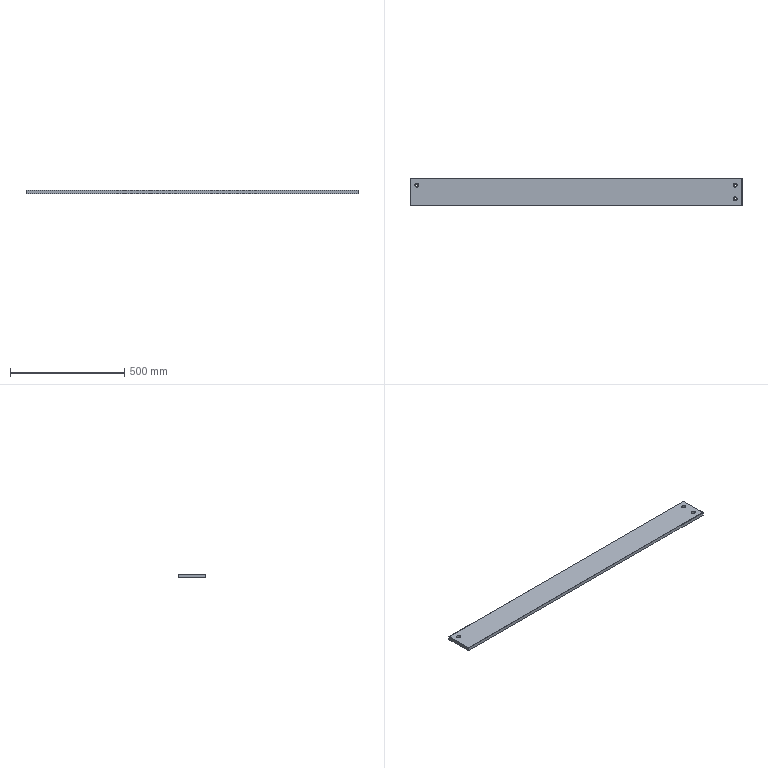Part | SolidWorks | features 3DProfileFeature 2, HoleWzd 2, Chamfer 1, Extrusion 1 | 1 solid | 25 faces | box 1453 x 120 x 15 mm | volume 2605469 mm3 | plane 13 | cylinder 12 | commonest cylinder face diameters 11 x6 18 x6
STEP:
#1=CARTESIAN_POINT('',(687.5,30.,-3.5));
#2=VERTEX_POINT('',#1);
#3=CARTESIAN_POINT('',(705.5,30.,-3.5));
#4=VERTEX_POINT('',#3);
#5=CARTESIAN_POINT('',(696.5,30.,-3.5));
#6=DIRECTION('',(0.,0.,1.));
#7=DIRECTION('',(1.,0.,0.));
#8=AXIS2_PLACEMENT_3D('',#5,#6,#7);
#9=CIRCLE('',#8,9.);
#10=EDGE_CURVE('',#2,#4,#9,.T.);
#11=ORIENTED_EDGE('',*,*,#10,.F.);
#12=CARTESIAN_POINT('',(687.5,30.,7.5));
#13=VERTEX_POINT('',#12);
#14=CARTESIAN_POINT('',(687.5,30.,7.5));
#15=DIRECTION('',(0.,0.,1.));
#16=VECTOR('',#15,1000.);
#17=LINE('',#14,#16);
#18=EDGE_CURVE('',#2,#13,#17,.T.);
#19=ORIENTED_EDGE('',*,*,#18,.T.);
#20=CARTESIAN_POINT('',(705.5,30.,7.5));
#21=VERTEX_POINT('',#20);
#22=CARTESIAN_POINT('',(696.5,30.,7.5));
#23=DIRECTION('',(0.,0.,1.));
#24=DIRECTION('',(1.,0.,0.));
#25=AXIS2_PLACEMENT_3D('',#22,#23,#24);
#26=CIRCLE('',#25,9.);
#27=EDGE_CURVE('',#13,#21,#26,.T.);
#28=ORIENTED_EDGE('',*,*,#27,.T.);
#29=CARTESIAN_POINT('',(705.5,30.,7.5));
#30=DIRECTION('',(0.,0.,1.));
#31=VECTOR('',#30,1000.);
#32=LINE('',#29,#31);
#33=EDGE_CURVE('',#4,#21,#32,.T.);
#34=ORIENTED_EDGE('',*,*,#33,.F.);
#35=EDGE_LOOP('',(#11,#19,#28,#34));
#36=FACE_OUTER_BOUND('',#35,.T.);
#37=CARTESIAN_POINT('',(696.5,30.,7.5));
#38=DIRECTION('',(0.,0.,1.));
#39=DIRECTION('',(1.,0.,0.));
#40=AXIS2_PLACEMENT_3D('',#37,#38,#39);
#41=CYLINDRICAL_SURFACE('',#40,9.);
#42=ADVANCED_FACE('',(#36),#41,.F.);
#43=CARTESIAN_POINT('',(691.,30.,-7.5));
#44=VERTEX_POINT('',#43);
#45=CARTESIAN_POINT('',(702.,30.,-7.5));
#46=VERTEX_POINT('',#45);
#47=CARTESIAN_POINT('',(696.5,30.,-7.5));
#48=DIRECTION('',(0.,0.,1.));
#49=DIRECTION('',(1.,0.,0.));
#50=AXIS2_PLACEMENT_3D('',#47,#48,#49);
#51=CIRCLE('',#50,5.5);
#52=EDGE_CURVE('',#44,#46,#51,.T.);
#53=ORIENTED_EDGE('',*,*,#52,.F.);
#54=CARTESIAN_POINT('',(691.,30.,-3.5));
#55=VERTEX_POINT('',#54);
#56=CARTESIAN_POINT('',(691.,30.,7.5));
#57=DIRECTION('',(0.,0.,1.));
#58=VECTOR('',#57,1000.);
#59=LINE('',#56,#58);
#60=EDGE_CURVE('',#44,#55,#59,.T.);
#61=ORIENTED_EDGE('',*,*,#60,.T.);
#62=CARTESIAN_POINT('',(702.,30.,-3.5));
#63=VERTEX_POINT('',#62);
#64=CARTESIAN_POINT('',(696.5,30.,-3.5));
#65=DIRECTION('',(0.,0.,1.));
#66=DIRECTION('',(1.,0.,0.));
#67=AXIS2_PLACEMENT_3D('',#64,#65,#66);
#68=CIRCLE('',#67,5.5);
#69=EDGE_CURVE('',#55,#63,#68,.T.);
#70=ORIENTED_EDGE('',*,*,#69,.T.);
#71=CARTESIAN_POINT('',(702.,30.,7.5));
#72=DIRECTION('',(0.,0.,1.));
#73=VECTOR('',#72,1000.);
#74=LINE('',#71,#73);
#75=EDGE_CURVE('',#46,#63,#74,.T.);
#76=ORIENTED_EDGE('',*,*,#75,.F.);
#77=EDGE_LOOP('',(#53,#61,#70,#76));
#78=FACE_OUTER_BOUND('',#77,.T.);
#79=CARTESIAN_POINT('',(696.5,30.,7.5));
#80=DIRECTION('',(0.,0.,1.));
#81=DIRECTION('',(1.,0.,0.));
#82=AXIS2_PLACEMENT_3D('',#79,#80,#81);
#83=CYLINDRICAL_SURFACE('',#82,5.5);
#84=ADVANCED_FACE('',(#78),#83,.F.);
#85=CARTESIAN_POINT('',(687.5,-30.,-3.5));
#86=VERTEX_POINT('',#85);
#87=CARTESIAN_POINT('',(705.5,-30.,-3.5));
#88=VERTEX_POINT('',#87);
#89=CARTESIAN_POINT('',(696.5,-30.,-3.5));
#90=DIRECTION('',(0.,0.,1.));
#91=DIRECTION('',(1.,0.,0.));
#92=AXIS2_PLACEMENT_3D('',#89,#90,#91);
#93=CIRCLE('',#92,9.);
#94=EDGE_CURVE('',#86,#88,#93,.T.);
#95=ORIENTED_EDGE('',*,*,#94,.F.);
#96=CARTESIAN_POINT('',(687.5,-30.,7.5));
#97=VERTEX_POINT('',#96);
#98=CARTESIAN_POINT('',(687.5,-30.,7.5));
#99=DIRECTION('',(0.,0.,1.));
#100=VECTOR('',#99,1000.);
#101=LINE('',#98,#100);
#102=EDGE_CURVE('',#86,#97,#101,.T.);
#103=ORIENTED_EDGE('',*,*,#102,.T.);
#104=CARTESIAN_POINT('',(705.5,-30.,7.5));
#105=VERTEX_POINT('',#104);
#106=CARTESIAN_POINT('',(696.5,-30.,7.5));
#107=DIRECTION('',(0.,0.,1.));
#108=DIRECTION('',(1.,0.,0.));
#109=AXIS2_PLACEMENT_3D('',#106,#107,#108);
#110=CIRCLE('',#109,9.);
#111=EDGE_CURVE('',#97,#105,#110,.T.);
#112=ORIENTED_EDGE('',*,*,#111,.T.);
#113=CARTESIAN_POINT('',(705.5,-30.,7.5));
#114=DIRECTION('',(0.,0.,1.));
#115=VECTOR('',#114,1000.);
#116=LINE('',#113,#115);
#117=EDGE_CURVE('',#88,#105,#116,.T.);
#118=ORIENTED_EDGE('',*,*,#117,.F.);
#119=EDGE_LOOP('',(#95,#103,#112,#118));
#120=FACE_OUTER_BOUND('',#119,.T.);
#121=CARTESIAN_POINT('',(696.5,-30.,7.5));
#122=DIRECTION('',(0.,0.,1.));
#123=DIRECTION('',(1.,0.,0.));
#124=AXIS2_PLACEMENT_3D('',#121,#122,#123);
#125=CYLINDRICAL_SURFACE('',#124,9.);
#126=ADVANCED_FACE('',(#120),#125,.F.);
#127=CARTESIAN_POINT('',(691.,-30.,-7.5));
#128=VERTEX_POINT('',#127);
#129=CARTESIAN_POINT('',(702.,-30.,-7.5));
#130=VERTEX_POINT('',#129);
#131=CARTESIAN_POINT('',(696.5,-30.,-7.5));
#132=DIRECTION('',(0.,0.,1.));
#133=DIRECTION('',(1.,0.,0.));
#134=AXIS2_PLACEMENT_3D('',#131,#132,#133);
#135=CIRCLE('',#134,5.5);
#136=EDGE_CURVE('',#128,#130,#135,.T.);
#137=ORIENTED_EDGE('',*,*,#136,.F.);
#138=CARTESIAN_POINT('',(691.,-30.,-3.5));
#139=VERTEX_POINT('',#138);
#140=CARTESIAN_POINT('',(691.,-30.,7.5));
#141=DIRECTION('',(0.,0.,1.));
#142=VECTOR('',#141,1000.);
#143=LINE('',#140,#142);
#144=EDGE_CURVE('',#128,#139,#143,.T.);
#145=ORIENTED_EDGE('',*,*,#144,.T.);
#146=CARTESIAN_POINT('',(702.,-30.,-3.5));
#147=VERTEX_POINT('',#146);
#148=CARTESIAN_POINT('',(696.5,-30.,-3.5));
#149=DIRECTION('',(0.,0.,1.));
#150=DIRECTION('',(1.,0.,0.));
#151=AXIS2_PLACEMENT_3D('',#148,#149,#150);
#152=CIRCLE('',#151,5.5);
#153=EDGE_CURVE('',#139,#147,#152,.T.);
#154=ORIENTED_EDGE('',*,*,#153,.T.);
#155=CARTESIAN_POINT('',(702.,-30.,7.5));
#156=DIRECTION('',(0.,0.,1.));
#157=VECTOR('',#156,1000.);
#158=LINE('',#155,#157);
#159=EDGE_CURVE('',#130,#147,#158,.T.);
#160=ORIENTED_EDGE('',*,*,#159,.F.);
#161=EDGE_LOOP('',(#137,#145,#154,#160));
#162=FACE_OUTER_BOUND('',#161,.T.);
#163=CARTESIAN_POINT('',(696.5,-30.,7.5));
#164=DIRECTION('',(0.,0.,1.));
#165=DIRECTION('',(1.,0.,0.));
#166=AXIS2_PLACEMENT_3D('',#163,#164,#165);
#167=CYLINDRICAL_SURFACE('',#166,5.5);
#168=ADVANCED_FACE('',(#162),#167,.F.);
#169=CARTESIAN_POINT('',(-705.5,30.,-3.5));
#170=VERTEX_POINT('',#169);
#171=CARTESIAN_POINT('',(-687.5,30.,-3.5));
#172=VERTEX_POINT('',#171);
#173=CARTESIAN_POINT('',(-696.5,30.,-3.5));
#174=DIRECTION('',(0.,0.,1.));
#175=DIRECTION('',(1.,0.,0.));
#176=AXIS2_PLACEMENT_3D('',#173,#174,#175);
#177=CIRCLE('',#176,9.);
#178=EDGE_CURVE('',#170,#172,#177,.T.);
#179=ORIENTED_EDGE('',*,*,#178,.F.);
#180=CARTESIAN_POINT('',(-705.5,30.,7.5));
#181=VERTEX_POINT('',#180);
#182=CARTESIAN_POINT('',(-705.5,30.,7.5));
#183=DIRECTION('',(0.,0.,1.));
#184=VECTOR('',#183,1000.);
#185=LINE('',#182,#184);
#186=EDGE_CURVE('',#170,#181,#185,.T.);
#187=ORIENTED_EDGE('',*,*,#186,.T.);
#188=CARTESIAN_POINT('',(-687.5,30.,7.5));
#189=VERTEX_POINT('',#188);
#190=CARTESIAN_POINT('',(-696.5,30.,7.5));
#191=DIRECTION('',(0.,0.,1.));
#192=DIRECTION('',(1.,0.,0.));
#193=AXIS2_PLACEMENT_3D('',#190,#191,#192);
#194=CIRCLE('',#193,9.);
#195=EDGE_CURVE('',#181,#189,#194,.T.);
#196=ORIENTED_EDGE('',*,*,#195,.T.);
#197=CARTESIAN_POINT('',(-687.5,30.,7.5));
#198=DIRECTION('',(0.,0.,1.));
#199=VECTOR('',#198,1000.);
#200=LINE('',#197,#199);
#201=EDGE_CURVE('',#172,#189,#200,.T.);
#202=ORIENTED_EDGE('',*,*,#201,.F.);
#203=EDGE_LOOP('',(#179,#187,#196,#202));
#204=FACE_OUTER_BOUND('',#203,.T.);
#205=CARTESIAN_POINT('',(-696.5,30.,7.5));
#206=DIRECTION('',(0.,0.,1.));
#207=DIRECTION('',(1.,0.,0.));
#208=AXIS2_PLACEMENT_3D('',#205,#206,#207);
#209=CYLINDRICAL_SURFACE('',#208,9.);
#210=ADVANCED_FACE('',(#204),#209,.F.);
#211=CARTESIAN_POINT('',(-702.,30.,-7.5));
#212=VERTEX_POINT('',#211);
#213=CARTESIAN_POINT('',(-691.,30.,-7.5));
#214=VERTEX_POINT('',#213);
#215=CARTESIAN_POINT('',(-696.5,30.,-7.5));
#216=DIRECTION('',(0.,0.,1.));
#217=DIRECTION('',(1.,0.,0.));
#218=AXIS2_PLACEMENT_3D('',#215,#216,#217);
#219=CIRCLE('',#218,5.5);
#220=EDGE_CURVE('',#212,#214,#219,.T.);
#221=ORIENTED_EDGE('',*,*,#220,.F.);
#222=CARTESIAN_POINT('',(-702.,30.,-3.5));
#223=VERTEX_POINT('',#222);
#224=CARTESIAN_POINT('',(-702.,30.,7.5));
#225=DIRECTION('',(0.,0.,1.));
#226=VECTOR('',#225,1000.);
#227=LINE('',#224,#226);
#228=EDGE_CURVE('',#212,#223,#227,.T.);
#229=ORIENTED_EDGE('',*,*,#228,.T.);
#230=CARTESIAN_POINT('',(-691.,30.,-3.5));
#231=VERTEX_POINT('',#230);
#232=CARTESIAN_POINT('',(-696.5,30.,-3.5));
#233=DIRECTION('',(0.,0.,1.));
#234=DIRECTION('',(1.,0.,0.));
#235=AXIS2_PLACEMENT_3D('',#232,#233,#234);
#236=CIRCLE('',#235,5.5);
#237=EDGE_CURVE('',#223,#231,#236,.T.);
#238=ORIENTED_EDGE('',*,*,#237,.T.);
#239=CARTESIAN_POINT('',(-691.,30.,7.5));
#240=DIRECTION('',(0.,0.,1.));
#241=VECTOR('',#240,1000.);
#242=LINE('',#239,#241);
#243=EDGE_CURVE('',#214,#231,#242,.T.);
#244=ORIENTED_EDGE('',*,*,#243,.F.);
#245=EDGE_LOOP('',(#221,#229,#238,#244));
#246=FACE_OUTER_BOUND('',#245,.T.);
#247=CARTESIAN_POINT('',(-696.5,30.,7.5));
#248=DIRECTION('',(0.,0.,1.));
#249=DIRECTION('',(1.,0.,0.));
#250=AXIS2_PLACEMENT_3D('',#247,#248,#249);
#251=CYLINDRICAL_SURFACE('',#250,5.5);
#252=ADVANCED_FACE('',(#246),#251,.F.);
#253=CARTESIAN_POINT('',(726.5,60.,7.));
#254=VERTEX_POINT('',#253);
#255=CARTESIAN_POINT('',(726.5,60.,-7.5));
#256=VERTEX_POINT('',#255);
#257=CARTESIAN_POINT('',(726.5,60.,7.5));
#258=DIRECTION('',(0.,0.,-1.));
#259=VECTOR('',#258,1000.);
#260=LINE('',#257,#259);
#261=EDGE_CURVE('',#254,#256,#260,.T.);
#262=ORIENTED_EDGE('',*,*,#261,.F.);
#263=CARTESIAN_POINT('',(726.5,-60.,7.));
#264=VERTEX_POINT('',#263);
#265=CARTESIAN_POINT('',(726.5,-60.,7.));
#266=DIRECTION('',(0.,-1.,0.));
#267=VECTOR('',#266,1000.);
#268=LINE('',#265,#267);
#269=EDGE_CURVE('',#254,#264,#268,.T.);
#270=ORIENTED_EDGE('',*,*,#269,.T.);
#271=CARTESIAN_POINT('',(726.5,-60.,-7.5));
#272=VERTEX_POINT('',#271);
#273=CARTESIAN_POINT('',(726.5,-60.,7.5));
#274=DIRECTION('',(0.,0.,-1.));
#275=VECTOR('',#274,1000.);
#276=LINE('',#273,#275);
#277=EDGE_CURVE('',#264,#272,#276,.T.);
#278=ORIENTED_EDGE('',*,*,#277,.T.);
#279=CARTESIAN_POINT('',(726.5,60.,-7.5));
#280=DIRECTION('',(0.,1.,0.));
#281=VECTOR('',#280,1000.);
#282=LINE('',#279,#281);
#283=EDGE_CURVE('',#272,#256,#282,.T.);
#284=ORIENTED_EDGE('',*,*,#283,.T.);
#285=EDGE_LOOP('',(#262,#270,#278,#284));
#286=FACE_OUTER_BOUND('',#285,.T.);
#287=CARTESIAN_POINT('',(726.5,60.,7.5));
#288=DIRECTION('',(-1.,0.,0.));
#289=DIRECTION('',(0.,0.,1.));
#290=AXIS2_PLACEMENT_3D('',#287,#288,#289);
#291=PLANE('',#290);
#292=ADVANCED_FACE('',(#286),#291,.F.);
#293=CARTESIAN_POINT('',(-726.5,60.,7.));
#294=VERTEX_POINT('',#293);
#295=CARTESIAN_POINT('',(-726.5,60.,-7.5));
#296=VERTEX_POINT('',#295);
#297=CARTESIAN_POINT('',(-726.5,60.,7.5));
#298=DIRECTION('',(0.,0.,-1.));
#299=VECTOR('',#298,1000.);
#300=LINE('',#297,#299);
#301=EDGE_CURVE('',#294,#296,#300,.T.);
#302=ORIENTED_EDGE('',*,*,#301,.F.);
#303=CARTESIAN_POINT('',(726.5,60.,7.));
#304=DIRECTION('',(1.,0.,0.));
#305=VECTOR('',#304,1000.);
#306=LINE('',#303,#305);
#307=EDGE_CURVE('',#294,#254,#306,.T.);
#308=ORIENTED_EDGE('',*,*,#307,.T.);
#309=ORIENTED_EDGE('',*,*,#261,.T.);
#310=CARTESIAN_POINT('',(-726.5,60.,-7.5));
#311=DIRECTION('',(-1.,0.,0.));
#312=VECTOR('',#311,1000.);
#313=LINE('',#310,#312);
#314=EDGE_CURVE('',#256,#296,#313,.T.);
#315=ORIENTED_EDGE('',*,*,#314,.T.);
#316=EDGE_LOOP('',(#302,#308,#309,#315));
#317=FACE_OUTER_BOUND('',#316,.T.);
#318=CARTESIAN_POINT('',(-726.5,60.,7.5));
#319=DIRECTION('',(0.,-1.,0.));
#320=DIRECTION('',(0.,0.,-1.));
#321=AXIS2_PLACEMENT_3D('',#318,#319,#320);
#322=PLANE('',#321);
#323=ADVANCED_FACE('',(#317),#322,.F.);
#324=CARTESIAN_POINT('',(-726.5,-60.,7.));
#325=VERTEX_POINT('',#324);
#326=CARTESIAN_POINT('',(-726.5,-60.,-7.5));
#327=VERTEX_POINT('',#326);
#328=CARTESIAN_POINT('',(-726.5,-60.,7.5));
#329=DIRECTION('',(0.,0.,-1.));
#330=VECTOR('',#329,1000.);
#331=LINE('',#328,#330);
#332=EDGE_CURVE('',#325,#327,#331,.T.);
#333=ORIENTED_EDGE('',*,*,#332,.F.);
#334=CARTESIAN_POINT('',(-726.5,60.,7.));
#335=DIRECTION('',(0.,1.,0.));
#336=VECTOR('',#335,1000.);
#337=LINE('',#334,#336);
#338=EDGE_CURVE('',#325,#294,#337,.T.);
#339=ORIENTED_EDGE('',*,*,#338,.T.);
#340=ORIENTED_EDGE('',*,*,#301,.T.);
#341=CARTESIAN_POINT('',(-726.5,60.,-7.5));
#342=DIRECTION('',(0.,-1.,0.));
#343=VECTOR('',#342,1000.);
#344=LINE('',#341,#343);
#345=EDGE_CURVE('',#296,#327,#344,.T.);
#346=ORIENTED_EDGE('',*,*,#345,.T.);
#347=EDGE_LOOP('',(#333,#339,#340,#346));
#348=FACE_OUTER_BOUND('',#347,.T.);
#349=CARTESIAN_POINT('',(-726.5,60.,7.5));
#350=DIRECTION('',(1.,0.,0.));
#351=DIRECTION('',(0.,0.,-1.));
#352=AXIS2_PLACEMENT_3D('',#349,#350,#351);
#353=PLANE('',#352);
#354=ADVANCED_FACE('',(#348),#353,.F.);
#355=ORIENTED_EDGE('',*,*,#277,.F.);
#356=CARTESIAN_POINT('',(-726.5,-60.,7.));
#357=DIRECTION('',(-1.,0.,0.));
#358=VECTOR('',#357,1000.);
#359=LINE('',#356,#358);
#360=EDGE_CURVE('',#264,#325,#359,.T.);
#361=ORIENTED_EDGE('',*,*,#360,.T.);
#362=ORIENTED_EDGE('',*,*,#332,.T.);
#363=CARTESIAN_POINT('',(-726.5,-60.,-7.5));
#364=DIRECTION('',(1.,0.,0.));
#365=VECTOR('',#364,1000.);
#366=LINE('',#363,#365);
#367=EDGE_CURVE('',#327,#272,#366,.T.);
#368=ORIENTED_EDGE('',*,*,#367,.T.);
#369=EDGE_LOOP('',(#355,#361,#362,#368));
#370=FACE_OUTER_BOUND('',#369,.T.);
#371=CARTESIAN_POINT('',(-726.5,-60.,7.5));
#372=DIRECTION('',(0.,1.,0.));
#373=DIRECTION('',(0.,0.,1.));
#374=AXIS2_PLACEMENT_3D('',#371,#372,#373);
#375=PLANE('',#374);
#376=ADVANCED_FACE('',(#370),#375,.F.);
#377=CARTESIAN_POINT('',(-726.,-59.5,7.5));
#378=VERTEX_POINT('',#377);
#379=CARTESIAN_POINT('',(726.,-59.5,7.5));
#380=VERTEX_POINT('',#379);
#381=CARTESIAN_POINT('',(726.5,-59.5,7.5));
#382=DIRECTION('',(1.,0.,0.));
#383=VECTOR('',#382,1000.);
#384=LINE('',#381,#383);
#385=EDGE_CURVE('',#378,#380,#384,.T.);
#386=ORIENTED_EDGE('',*,*,#385,.T.);
#387=CARTESIAN_POINT('',(726.,59.5,7.5));
#388=VERTEX_POINT('',#387);
#389=CARTESIAN_POINT('',(726.,60.,7.5));
#390=DIRECTION('',(0.,1.,0.));
#391=VECTOR('',#390,1000.);
#392=LINE('',#389,#391);
#393=EDGE_CURVE('',#380,#388,#392,.T.);
#394=ORIENTED_EDGE('',*,*,#393,.T.);
#395=CARTESIAN_POINT('',(-726.,59.5,7.5));
#396=VERTEX_POINT('',#395);
#397=CARTESIAN_POINT('',(-726.5,59.5,7.5));
#398=DIRECTION('',(-1.,0.,0.));
#399=VECTOR('',#398,1000.);
#400=LINE('',#397,#399);
#401=EDGE_CURVE('',#388,#396,#400,.T.);
#402=ORIENTED_EDGE('',*,*,#401,.T.);
#403=CARTESIAN_POINT('',(-726.,-60.,7.5));
#404=DIRECTION('',(0.,-1.,0.));
#405=VECTOR('',#404,1000.);
#406=LINE('',#403,#405);
#407=EDGE_CURVE('',#396,#378,#406,.T.);
#408=ORIENTED_EDGE('',*,*,#407,.T.);
#409=EDGE_LOOP('',(#386,#394,#402,#408));
#410=FACE_OUTER_BOUND('',#409,.T.);
#411=CARTESIAN_POINT('',(696.5,30.,7.5));
#412=DIRECTION('',(0.,0.,1.));
#413=DIRECTION('',(1.,0.,0.));
#414=AXIS2_PLACEMENT_3D('',#411,#412,#413);
#415=CIRCLE('',#414,9.);
#416=EDGE_CURVE('',#21,#13,#415,.T.);
#417=ORIENTED_EDGE('',*,*,#416,.F.);
#418=ORIENTED_EDGE('',*,*,#27,.F.);
#419=EDGE_LOOP('',(#417,#418));
#420=FACE_BOUND('',#419,.T.);
#421=CARTESIAN_POINT('',(696.5,-30.,7.5));
#422=DIRECTION('',(0.,0.,1.));
#423=DIRECTION('',(1.,0.,0.));
#424=AXIS2_PLACEMENT_3D('',#421,#422,#423);
#425=CIRCLE('',#424,9.);
#426=EDGE_CURVE('',#105,#97,#425,.T.);
#427=ORIENTED_EDGE('',*,*,#426,.F.);
#428=ORIENTED_EDGE('',*,*,#111,.F.);
#429=EDGE_LOOP('',(#427,#428));
#430=FACE_BOUND('',#429,.T.);
#431=CARTESIAN_POINT('',(-696.5,30.,7.5));
#432=DIRECTION('',(0.,0.,1.));
#433=DIRECTION('',(1.,0.,0.));
#434=AXIS2_PLACEMENT_3D('',#431,#432,#433);
#435=CIRCLE('',#434,9.);
#436=EDGE_CURVE('',#189,#181,#435,.T.);
#437=ORIENTED_EDGE('',*,*,#436,.F.);
#438=ORIENTED_EDGE('',*,*,#195,.F.);
#439=EDGE_LOOP('',(#437,#438));
#440=FACE_BOUND('',#439,.T.);
#441=CARTESIAN_POINT('',(0.,0.,7.5));
#442=DIRECTION('',(0.,0.,1.));
#443=DIRECTION('',(1.,0.,0.));
#444=AXIS2_PLACEMENT_3D('',#441,#442,#443);
#445=PLANE('',#444);
#446=ADVANCED_FACE('',(#410,#420,#430,#440),#445,.T.);
#447=CARTESIAN_POINT('',(696.5,30.,-7.5));
#448=DIRECTION('',(0.,0.,1.));
#449=DIRECTION('',(1.,0.,0.));
#450=AXIS2_PLACEMENT_3D('',#447,#448,#449);
#451=CIRCLE('',#450,5.5);
#452=EDGE_CURVE('',#46,#44,#451,.T.);
#453=ORIENTED_EDGE('',*,*,#452,.T.);
#454=ORIENTED_EDGE('',*,*,#52,.T.);
#455=EDGE_LOOP('',(#453,#454));
#456=FACE_BOUND('',#455,.T.);
#457=CARTESIAN_POINT('',(696.5,-30.,-7.5));
#458=DIRECTION('',(0.,0.,1.));
#459=DIRECTION('',(1.,0.,0.));
#460=AXIS2_PLACEMENT_3D('',#457,#458,#459);
#461=CIRCLE('',#460,5.5);
#462=EDGE_CURVE('',#130,#128,#461,.T.);
#463=ORIENTED_EDGE('',*,*,#462,.T.);
#464=ORIENTED_EDGE('',*,*,#136,.T.);
#465=EDGE_LOOP('',(#463,#464));
#466=FACE_BOUND('',#465,.T.);
#467=CARTESIAN_POINT('',(-696.5,30.,-7.5));
#468=DIRECTION('',(0.,0.,1.));
#469=DIRECTION('',(1.,0.,0.));
#470=AXIS2_PLACEMENT_3D('',#467,#468,#469);
#471=CIRCLE('',#470,5.5);
#472=EDGE_CURVE('',#214,#212,#471,.T.);
#473=ORIENTED_EDGE('',*,*,#472,.T.);
#474=ORIENTED_EDGE('',*,*,#220,.T.);
#475=EDGE_LOOP('',(#473,#474));
#476=FACE_BOUND('',#475,.T.);
#477=ORIENTED_EDGE('',*,*,#283,.F.);
#478=ORIENTED_EDGE('',*,*,#367,.F.);
#479=ORIENTED_EDGE('',*,*,#345,.F.);
#480=ORIENTED_EDGE('',*,*,#314,.F.);
#481=EDGE_LOOP('',(#477,#478,#479,#480));
#482=FACE_OUTER_BOUND('',#481,.T.);
#483=CARTESIAN_POINT('',(0.,0.,-7.5));
#484=DIRECTION('',(0.,0.,1.));
#485=DIRECTION('',(1.,0.,0.));
#486=AXIS2_PLACEMENT_3D('',#483,#484,#485);
#487=PLANE('',#486);
#488=ADVANCED_FACE('',(#456,#466,#476,#482),#487,.F.);
#489=ORIENTED_EDGE('',*,*,#228,.F.);
#490=ORIENTED_EDGE('',*,*,#472,.F.);
#491=ORIENTED_EDGE('',*,*,#243,.T.);
#492=CARTESIAN_POINT('',(-696.5,30.,-3.5));
#493=DIRECTION('',(0.,0.,1.));
#494=DIRECTION('',(1.,0.,0.));
#495=AXIS2_PLACEMENT_3D('',#492,#493,#494);
#496=CIRCLE('',#495,5.5);
#497=EDGE_CURVE('',#231,#223,#496,.T.);
#498=ORIENTED_EDGE('',*,*,#497,.T.);
#499=EDGE_LOOP('',(#489,#490,#491,#498));
#500=FACE_OUTER_BOUND('',#499,.T.);
#501=CARTESIAN_POINT('',(-696.5,30.,7.5));
#502=DIRECTION('',(0.,0.,1.));
#503=DIRECTION('',(1.,0.,0.));
#504=AXIS2_PLACEMENT_3D('',#501,#502,#503);
#505=CYLINDRICAL_SURFACE('',#504,5.5);
#506=ADVANCED_FACE('',(#500),#505,.F.);
#507=ORIENTED_EDGE('',*,*,#497,.F.);
#508=ORIENTED_EDGE('',*,*,#237,.F.);
#509=EDGE_LOOP('',(#507,#508));
#510=FACE_BOUND('',#509,.T.);
#511=CARTESIAN_POINT('',(-696.5,30.,-3.5));
#512=DIRECTION('',(0.,0.,1.));
#513=DIRECTION('',(1.,0.,0.));
#514=AXIS2_PLACEMENT_3D('',#511,#512,#513);
#515=CIRCLE('',#514,9.);
#516=EDGE_CURVE('',#172,#170,#515,.T.);
#517=ORIENTED_EDGE('',*,*,#516,.T.);
#518=ORIENTED_EDGE('',*,*,#178,.T.);
#519=EDGE_LOOP('',(#517,#518));
#520=FACE_OUTER_BOUND('',#519,.T.);
#521=CARTESIAN_POINT('',(-691.,30.,-3.5));
#522=DIRECTION('',(0.,0.,-1.));
#523=DIRECTION('',(-1.,0.,0.));
#524=AXIS2_PLACEMENT_3D('',#521,#522,#523);
#525=PLANE('',#524);
#526=ADVANCED_FACE('',(#510,#520),#525,.F.);
#527=ORIENTED_EDGE('',*,*,#186,.F.);
#528=ORIENTED_EDGE('',*,*,#516,.F.);
#529=ORIENTED_EDGE('',*,*,#201,.T.);
#530=ORIENTED_EDGE('',*,*,#436,.T.);
#531=EDGE_LOOP('',(#527,#528,#529,#530));
#532=FACE_OUTER_BOUND('',#531,.T.);
#533=CARTESIAN_POINT('',(-696.5,30.,7.5));
#534=DIRECTION('',(0.,0.,1.));
#535=DIRECTION('',(1.,0.,0.));
#536=AXIS2_PLACEMENT_3D('',#533,#534,#535);
#537=CYLINDRICAL_SURFACE('',#536,9.);
#538=ADVANCED_FACE('',(#532),#537,.F.);
#539=ORIENTED_EDGE('',*,*,#144,.F.);
#540=ORIENTED_EDGE('',*,*,#462,.F.);
#541=ORIENTED_EDGE('',*,*,#159,.T.);
#542=CARTESIAN_POINT('',(696.5,-30.,-3.5));
#543=DIRECTION('',(0.,0.,1.));
#544=DIRECTION('',(1.,0.,0.));
#545=AXIS2_PLACEMENT_3D('',#542,#543,#544);
#546=CIRCLE('',#545,5.5);
#547=EDGE_CURVE('',#147,#139,#546,.T.);
#548=ORIENTED_EDGE('',*,*,#547,.T.);
#549=EDGE_LOOP('',(#539,#540,#541,#548));
#550=FACE_OUTER_BOUND('',#549,.T.);
#551=CARTESIAN_POINT('',(696.5,-30.,7.5));
#552=DIRECTION('',(0.,0.,1.));
#553=DIRECTION('',(1.,0.,0.));
#554=AXIS2_PLACEMENT_3D('',#551,#552,#553);
#555=CYLINDRICAL_SURFACE('',#554,5.5);
#556=ADVANCED_FACE('',(#550),#555,.F.);
#557=ORIENTED_EDGE('',*,*,#547,.F.);
#558=ORIENTED_EDGE('',*,*,#153,.F.);
#559=EDGE_LOOP('',(#557,#558));
#560=FACE_BOUND('',#559,.T.);
#561=CARTESIAN_POINT('',(696.5,-30.,-3.5));
#562=DIRECTION('',(0.,0.,1.));
#563=DIRECTION('',(1.,0.,0.));
#564=AXIS2_PLACEMENT_3D('',#561,#562,#563);
#565=CIRCLE('',#564,9.);
#566=EDGE_CURVE('',#88,#86,#565,.T.);
#567=ORIENTED_EDGE('',*,*,#566,.T.);
#568=ORIENTED_EDGE('',*,*,#94,.T.);
#569=EDGE_LOOP('',(#567,#568));
#570=FACE_OUTER_BOUND('',#569,.T.);
#571=CARTESIAN_POINT('',(702.,-30.,-3.5));
#572=DIRECTION('',(0.,0.,-1.));
#573=DIRECTION('',(-1.,0.,0.));
#574=AXIS2_PLACEMENT_3D('',#571,#572,#573);
#575=PLANE('',#574);
#576=ADVANCED_FACE('',(#560,#570),#575,.F.);
#577=ORIENTED_EDGE('',*,*,#102,.F.);
#578=ORIENTED_EDGE('',*,*,#566,.F.);
#579=ORIENTED_EDGE('',*,*,#117,.T.);
#580=ORIENTED_EDGE('',*,*,#426,.T.);
#581=EDGE_LOOP('',(#577,#578,#579,#580));
#582=FACE_OUTER_BOUND('',#581,.T.);
#583=CARTESIAN_POINT('',(696.5,-30.,7.5));
#584=DIRECTION('',(0.,0.,1.));
#585=DIRECTION('',(1.,0.,0.));
#586=AXIS2_PLACEMENT_3D('',#583,#584,#585);
#587=CYLINDRICAL_SURFACE('',#586,9.);
#588=ADVANCED_FACE('',(#582),#587,.F.);
#589=ORIENTED_EDGE('',*,*,#60,.F.);
#590=ORIENTED_EDGE('',*,*,#452,.F.);
#591=ORIENTED_EDGE('',*,*,#75,.T.);
#592=CARTESIAN_POINT('',(696.5,30.,-3.5));
#593=DIRECTION('',(0.,0.,1.));
#594=DIRECTION('',(1.,0.,0.));
#595=AXIS2_PLACEMENT_3D('',#592,#593,#594);
#596=CIRCLE('',#595,5.5);
#597=EDGE_CURVE('',#63,#55,#596,.T.);
#598=ORIENTED_EDGE('',*,*,#597,.T.);
#599=EDGE_LOOP('',(#589,#590,#591,#598));
#600=FACE_OUTER_BOUND('',#599,.T.);
#601=CARTESIAN_POINT('',(696.5,30.,7.5));
#602=DIRECTION('',(0.,0.,1.));
#603=DIRECTION('',(1.,0.,0.));
#604=AXIS2_PLACEMENT_3D('',#601,#602,#603);
#605=CYLINDRICAL_SURFACE('',#604,5.5);
#606=ADVANCED_FACE('',(#600),#605,.F.);
#607=ORIENTED_EDGE('',*,*,#597,.F.);
#608=ORIENTED_EDGE('',*,*,#69,.F.);
#609=EDGE_LOOP('',(#607,#608));
#610=FACE_BOUND('',#609,.T.);
#611=CARTESIAN_POINT('',(696.5,30.,-3.5));
#612=DIRECTION('',(0.,0.,1.));
#613=DIRECTION('',(1.,0.,0.));
#614=AXIS2_PLACEMENT_3D('',#611,#612,#613);
#615=CIRCLE('',#614,9.);
#616=EDGE_CURVE('',#4,#2,#615,.T.);
#617=ORIENTED_EDGE('',*,*,#616,.T.);
#618=ORIENTED_EDGE('',*,*,#10,.T.);
#619=EDGE_LOOP('',(#617,#618));
#620=FACE_OUTER_BOUND('',#619,.T.);
#621=CARTESIAN_POINT('',(702.,30.,-3.5));
#622=DIRECTION('',(0.,0.,-1.));
#623=DIRECTION('',(-1.,0.,0.));
#624=AXIS2_PLACEMENT_3D('',#621,#622,#623);
#625=PLANE('',#624);
#626=ADVANCED_FACE('',(#610,#620),#625,.F.);
#627=ORIENTED_EDGE('',*,*,#18,.F.);
#628=ORIENTED_EDGE('',*,*,#616,.F.);
#629=ORIENTED_EDGE('',*,*,#33,.T.);
#630=ORIENTED_EDGE('',*,*,#416,.T.);
#631=EDGE_LOOP('',(#627,#628,#629,#630));
#632=FACE_OUTER_BOUND('',#631,.T.);
#633=CARTESIAN_POINT('',(696.5,30.,7.5));
#634=DIRECTION('',(0.,0.,1.));
#635=DIRECTION('',(1.,0.,0.));
#636=AXIS2_PLACEMENT_3D('',#633,#634,#635);
#637=CYLINDRICAL_SURFACE('',#636,9.);
#638=ADVANCED_FACE('',(#632),#637,.F.);
#639=CARTESIAN_POINT('',(-484.,-182.5,249.5));
#640=DIRECTION('',(0.5774,-0.5774,0.5774));
#641=VECTOR('',#640,1000.);
#642=LINE('',#639,#641);
#643=EDGE_CURVE('',#294,#396,#642,.T.);
#644=ORIENTED_EDGE('',*,*,#643,.F.);
#645=ORIENTED_EDGE('',*,*,#338,.F.);
#646=CARTESIAN_POINT('',(-706.167,-39.667,27.333));
#647=DIRECTION('',(-0.5774,-0.5774,-0.5774));
#648=VECTOR('',#647,1000.);
#649=LINE('',#646,#648);
#650=EDGE_CURVE('',#378,#325,#649,.T.);
#651=ORIENTED_EDGE('',*,*,#650,.F.);
#652=ORIENTED_EDGE('',*,*,#407,.F.);
#653=EDGE_LOOP('',(#644,#645,#651,#652));
#654=FACE_OUTER_BOUND('',#653,.T.);
#655=CARTESIAN_POINT('',(-726.,0.,7.5));
#656=DIRECTION('',(-0.7071,0.,0.7071));
#657=DIRECTION('',(0.,1.,0.));
#658=AXIS2_PLACEMENT_3D('',#655,#656,#657);
#659=PLANE('',#658);
#660=ADVANCED_FACE('',(#654),#659,.T.);
#661=ORIENTED_EDGE('',*,*,#650,.T.);
#662=ORIENTED_EDGE('',*,*,#360,.F.);
#663=CARTESIAN_POINT('',(484.,182.5,249.5));
#664=DIRECTION('',(0.5774,-0.5774,-0.5774));
#665=VECTOR('',#664,1000.);
#666=LINE('',#663,#665);
#667=EDGE_CURVE('',#380,#264,#666,.T.);
#668=ORIENTED_EDGE('',*,*,#667,.F.);
#669=ORIENTED_EDGE('',*,*,#385,.F.);
#670=EDGE_LOOP('',(#661,#662,#668,#669));
#671=FACE_OUTER_BOUND('',#670,.T.);
#672=CARTESIAN_POINT('',(0.,-59.5,7.5));
#673=DIRECTION('',(0.,-0.7071,0.7071));
#674=DIRECTION('',(-1.,0.,0.));
#675=AXIS2_PLACEMENT_3D('',#672,#673,#674);
#676=PLANE('',#675);
#677=ADVANCED_FACE('',(#671),#676,.T.);
#678=ORIENTED_EDGE('',*,*,#643,.T.);
#679=ORIENTED_EDGE('',*,*,#401,.F.);
#680=CARTESIAN_POINT('',(484.,-182.5,249.5));
#681=DIRECTION('',(-0.5774,-0.5774,0.5774));
#682=VECTOR('',#681,1000.);
#683=LINE('',#680,#682);
#684=EDGE_CURVE('',#254,#388,#683,.T.);
#685=ORIENTED_EDGE('',*,*,#684,.F.);
#686=ORIENTED_EDGE('',*,*,#307,.F.);
#687=EDGE_LOOP('',(#678,#679,#685,#686));
#688=FACE_OUTER_BOUND('',#687,.T.);
#689=CARTESIAN_POINT('',(0.,59.5,7.5));
#690=DIRECTION('',(0.,0.7071,0.7071));
#691=DIRECTION('',(1.,0.,0.));
#692=AXIS2_PLACEMENT_3D('',#689,#690,#691);
#693=PLANE('',#692);
#694=ADVANCED_FACE('',(#688),#693,.T.);
#695=ORIENTED_EDGE('',*,*,#667,.T.);
#696=ORIENTED_EDGE('',*,*,#269,.F.);
#697=ORIENTED_EDGE('',*,*,#684,.T.);
#698=ORIENTED_EDGE('',*,*,#393,.F.);
#699=EDGE_LOOP('',(#695,#696,#697,#698));
#700=FACE_OUTER_BOUND('',#699,.T.);
#701=CARTESIAN_POINT('',(726.,0.,7.5));
#702=DIRECTION('',(0.7071,0.,0.7071));
#703=DIRECTION('',(0.,-1.,0.));
#704=AXIS2_PLACEMENT_3D('',#701,#702,#703);
#705=PLANE('',#704);
#706=ADVANCED_FACE('',(#700),#705,.T.);
#707=CLOSED_SHELL('',(#42,#84,#126,#168,#210,#252,#292,#323,#354,#376,#446,#488,#506,#526,#538,#556,#576,#588,#606,#626,#638,#660,#677,#694,#706));
#708=MANIFOLD_SOLID_BREP('',#707);
#709=CARTESIAN_POINT('',(0.,0.,0.));
#710=DIRECTION('',(0.,0.,1.));
#711=DIRECTION('',(1.,0.,0.));
#712=AXIS2_PLACEMENT_3D('',#709,#710,#711);
#713=(LENGTH_UNIT()NAMED_UNIT(*)SI_UNIT(.MILLI.,.METRE.));
#714=UNCERTAINTY_MEASURE_WITH_UNIT(LENGTH_MEASURE(0.00001),#713,'','');
#715=(NAMED_UNIT(*)PLANE_ANGLE_UNIT()SI_UNIT($,.RADIAN.));
#716=(NAMED_UNIT(*)SI_UNIT($,.STERADIAN.)SOLID_ANGLE_UNIT());
#717=(GEOMETRIC_REPRESENTATION_CONTEXT(3)GLOBAL_UNCERTAINTY_ASSIGNED_CONTEXT((#714))GLOBAL_UNIT_ASSIGNED_CONTEXT((#713,#715,#716))REPRESENTATION_CONTEXT('',''));
#718=ADVANCED_BREP_SHAPE_REPRESENTATION('',(#708,#712),#717);